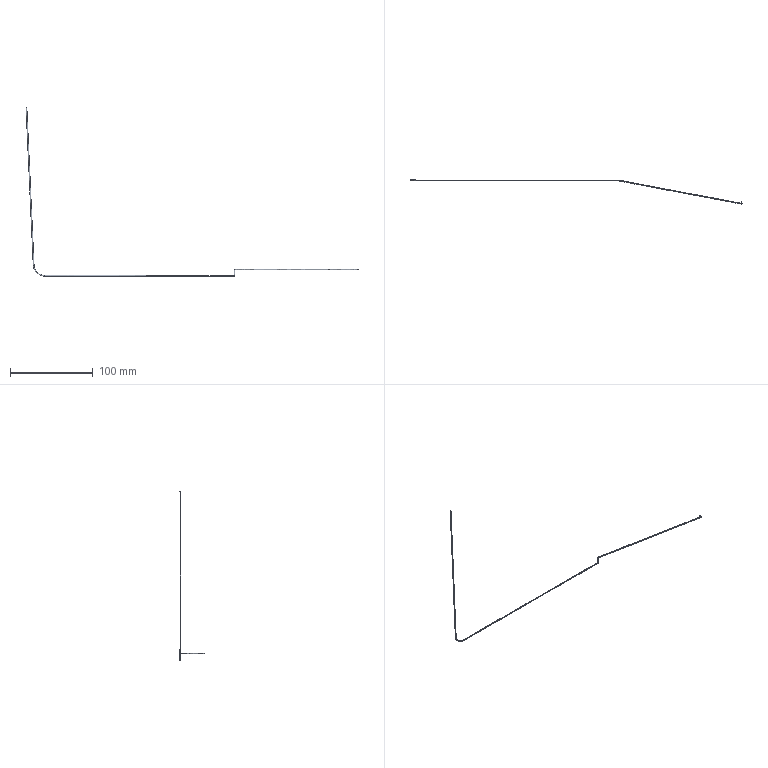Part | SolidWorks | features 3DProfileFeature 4, Sweep 1 | 1 solid | 14 faces | box 401.907 x 29.216 x 204.55 mm | volume 473.935 mm3 | spline 12 | plane 2
STEP:
#1=CARTESIAN_POINT('',(-84.907,75.023,0.4908));
#2=VERTEX_POINT('',#1);
#3=CARTESIAN_POINT('',(-85.093,74.977,-0.4908));
#4=VERTEX_POINT('',#3);
#5=CARTESIAN_POINT('',(-85.,75.,0.));
#6=DIRECTION('',(0.008513,-0.9989,0.04512));
#7=DIRECTION('',(0.1852,0.04591,0.9816));
#8=AXIS2_PLACEMENT_3D('',#5,#6,#7);
#9=CIRCLE('',#8,0.5);
#10=EDGE_CURVE('',#2,#4,#9,.T.);
#11=ORIENTED_EDGE('',*,*,#10,.T.);
#12=CARTESIAN_POINT('',(-85.093,71.998,-0.4908));
#13=VERTEX_POINT('',#12);
#14=CARTESIAN_POINT('',(-85.093,74.977,-0.4908));
#15=CARTESIAN_POINT('',(-85.093,71.998,-0.4908));
#16=B_SPLINE_CURVE_WITH_KNOTS('',1,(#14,#15),.UNSPECIFIED.,.F.,.F.,(2,2),(0.,0.6385),.UNSPECIFIED.);
#17=EDGE_CURVE('',#4,#13,#16,.T.);
#18=ORIENTED_EDGE('',*,*,#17,.T.);
#19=CARTESIAN_POINT('',(-84.907,71.775,0.4908));
#20=VERTEX_POINT('',#19);
#21=CARTESIAN_POINT('',(-85.093,71.998,-0.4908));
#22=CARTESIAN_POINT('',(-85.147,72.063,-0.4806));
#23=CARTESIAN_POINT('',(-85.199,72.127,-0.4617));
#24=CARTESIAN_POINT('',(-85.3,72.248,-0.4037));
#25=CARTESIAN_POINT('',(-85.349,72.307,-0.3639));
#26=CARTESIAN_POINT('',(-85.434,72.41,-0.2574));
#27=CARTESIAN_POINT('',(-85.47,72.454,-0.1886));
#28=CARTESIAN_POINT('',(-85.506,72.497,-0.02785));
#29=CARTESIAN_POINT('',(-85.502,72.492,0.06372));
#30=CARTESIAN_POINT('',(-85.457,72.437,0.2187));
#31=CARTESIAN_POINT('',(-85.418,72.39,0.2827));
#32=CARTESIAN_POINT('',(-85.33,72.284,0.3816));
#33=CARTESIAN_POINT('',(-85.28,72.224,0.4182));
#34=CARTESIAN_POINT('',(-85.126,72.038,0.4971));
#35=CARTESIAN_POINT('',(-85.015,71.905,0.5112));
#36=CARTESIAN_POINT('',(-84.907,71.775,0.4908));
#37=B_SPLINE_CURVE_WITH_KNOTS('',3,(#21,#22,#23,#24,#25,#26,#27,#28,#29,#30,#31,#32,#33,#34,#35,#36),.UNSPECIFIED.,.F.,.F.,(4,2,2,2,2,2,2,4),(0.002044,0.0023,0.002555,0.002811,0.003067,0.003322,0.003578,0.004089),.UNSPECIFIED.);
#38=EDGE_CURVE('',#13,#20,#37,.T.);
#39=ORIENTED_EDGE('',*,*,#38,.T.);
#40=CARTESIAN_POINT('',(-84.907,75.023,0.4908));
#41=CARTESIAN_POINT('',(-84.907,71.775,0.4908));
#42=B_SPLINE_CURVE_WITH_KNOTS('',1,(#40,#41),.UNSPECIFIED.,.F.,.F.,(2,2),(0.,0.6962),.UNSPECIFIED.);
#43=EDGE_CURVE('',#2,#20,#42,.T.);
#44=ORIENTED_EDGE('',*,*,#43,.F.);
#45=EDGE_LOOP('',(#11,#18,#39,#44));
#46=FACE_OUTER_BOUND('',#45,.T.);
#47=CARTESIAN_POINT('',(-84.907,75.023,0.4908));
#48=CARTESIAN_POINT('',(-84.907,70.357,0.4908));
#49=CARTESIAN_POINT('',(-85.89,75.023,0.6762));
#50=CARTESIAN_POINT('',(-85.89,70.357,0.6762));
#51=CARTESIAN_POINT('',(-86.075,74.977,-0.3054));
#52=CARTESIAN_POINT('',(-86.075,70.311,-0.3054));
#53=CARTESIAN_POINT('',(-85.093,74.977,-0.4908));
#54=CARTESIAN_POINT('',(-85.093,70.311,-0.4908));
#55=CARTESIAN_POINT('',(-84.11,74.977,-0.6762));
#56=CARTESIAN_POINT('',(-84.11,70.311,-0.6762));
#57=CARTESIAN_POINT('',(-83.925,75.023,0.3054));
#58=CARTESIAN_POINT('',(-83.925,70.357,0.3054));
#59=CARTESIAN_POINT('',(-84.907,75.023,0.4908));
#60=CARTESIAN_POINT('',(-84.907,70.357,0.4908));
#61=(BOUNDED_SURFACE()B_SPLINE_SURFACE(3,1,((#47,#48),(#49,#50),(#51,#52),(#53,#54),(#55,#56),(#57,#58),(#59,#60)),.UNSPECIFIED.,.T.,.F.,.T.)B_SPLINE_SURFACE_WITH_KNOTS((4,3,4),(2,2),(0.,0.5,1.),(0.,1.),.UNSPECIFIED.)GEOMETRIC_REPRESENTATION_ITEM()RATIONAL_B_SPLINE_SURFACE(((1.,1.),(0.3333,0.3333),(0.3333,0.3333),(1.,1.),(0.3333,0.3333),(0.3333,0.3333),(1.,1.)))REPRESENTATION_ITEM('')SURFACE());
#62=ADVANCED_FACE('',(#46),#61,.T.);
#63=ORIENTED_EDGE('',*,*,#38,.F.);
#64=CARTESIAN_POINT('',(-233.501,100.,-0.4908));
#65=VERTEX_POINT('',#64);
#66=CARTESIAN_POINT('',(-85.093,71.998,-0.4908));
#67=CARTESIAN_POINT('',(-233.501,100.,-0.4908));
#68=B_SPLINE_CURVE_WITH_KNOTS('',1,(#66,#67),.UNSPECIFIED.,.F.,.F.,(2,2),(0.01033,0.991),.UNSPECIFIED.);
#69=EDGE_CURVE('',#13,#65,#68,.T.);
#70=ORIENTED_EDGE('',*,*,#69,.T.);
#71=CARTESIAN_POINT('',(-234.499,100.,0.4908));
#72=VERTEX_POINT('',#71);
#73=CARTESIAN_POINT('',(-233.501,100.,-0.4908));
#74=CARTESIAN_POINT('',(-233.501,100.078,-0.4763));
#75=CARTESIAN_POINT('',(-233.52,100.153,-0.4438));
#76=CARTESIAN_POINT('',(-233.578,100.277,-0.3631));
#77=CARTESIAN_POINT('',(-233.618,100.328,-0.3145));
#78=CARTESIAN_POINT('',(-233.751,100.45,-0.1609));
#79=CARTESIAN_POINT('',(-233.86,100.493,-0.04587));
#80=CARTESIAN_POINT('',(-234.03,100.502,0.1222));
#81=CARTESIAN_POINT('',(-234.086,100.496,0.1766));
#82=CARTESIAN_POINT('',(-234.199,100.462,0.2817));
#83=CARTESIAN_POINT('',(-234.256,100.434,0.3323));
#84=CARTESIAN_POINT('',(-234.361,100.352,0.4199));
#85=CARTESIAN_POINT('',(-234.409,100.297,0.4572));
#86=CARTESIAN_POINT('',(-234.479,100.16,0.5007));
#87=CARTESIAN_POINT('',(-234.499,100.079,0.5055));
#88=CARTESIAN_POINT('',(-234.499,100.,0.4908));
#89=B_SPLINE_CURVE_WITH_KNOTS('',3,(#73,#74,#75,#76,#77,#78,#79,#80,#81,#82,#83,#84,#85,#86,#87,#88),.UNSPECIFIED.,.F.,.F.,(4,2,2,2,2,2,2,4),(0.001901,0.002138,0.002375,0.00285,0.003087,0.003324,0.003562,0.003799),.UNSPECIFIED.);
#90=EDGE_CURVE('',#65,#72,#89,.T.);
#91=ORIENTED_EDGE('',*,*,#90,.T.);
#92=CARTESIAN_POINT('',(-84.907,71.775,0.4908));
#93=CARTESIAN_POINT('',(-234.499,100.,0.4908));
#94=B_SPLINE_CURVE_WITH_KNOTS('',1,(#92,#93),.UNSPECIFIED.,.F.,.F.,(2,2),(0.009174,0.9977),.UNSPECIFIED.);
#95=EDGE_CURVE('',#20,#72,#94,.T.);
#96=ORIENTED_EDGE('',*,*,#95,.F.);
#97=EDGE_LOOP('',(#63,#70,#91,#96));
#98=FACE_OUTER_BOUND('',#97,.T.);
#99=CARTESIAN_POINT('',(-83.519,71.513,0.4908));
#100=CARTESIAN_POINT('',(-234.849,100.066,0.4908));
#101=CARTESIAN_POINT('',(-83.337,72.478,0.6762));
#102=CARTESIAN_POINT('',(-234.666,101.032,0.6762));
#103=CARTESIAN_POINT('',(-83.348,72.669,-0.3054));
#104=CARTESIAN_POINT('',(-234.677,101.222,-0.3054));
#105=CARTESIAN_POINT('',(-83.53,71.703,-0.4908));
#106=CARTESIAN_POINT('',(-234.859,100.256,-0.4908));
#107=CARTESIAN_POINT('',(-83.712,70.738,-0.6762));
#108=CARTESIAN_POINT('',(-235.042,99.291,-0.6762));
#109=CARTESIAN_POINT('',(-83.701,70.547,0.3054));
#110=CARTESIAN_POINT('',(-235.031,99.1,0.3054));
#111=CARTESIAN_POINT('',(-83.519,71.513,0.4908));
#112=CARTESIAN_POINT('',(-234.849,100.066,0.4908));
#113=(BOUNDED_SURFACE()B_SPLINE_SURFACE(3,1,((#99,#100),(#101,#102),(#103,#104),(#105,#106),(#107,#108),(#109,#110),(#111,#112)),.UNSPECIFIED.,.T.,.F.,.F.)B_SPLINE_SURFACE_WITH_KNOTS((4,3,4),(2,2),(0.,0.5,1.),(0.,1.),.UNSPECIFIED.)GEOMETRIC_REPRESENTATION_ITEM()RATIONAL_B_SPLINE_SURFACE(((1.,1.),(0.3333,0.3333),(0.3333,0.3333),(1.,1.),(0.3333,0.3333),(0.3333,0.3333),(1.,1.)))REPRESENTATION_ITEM('')SURFACE());
#114=ADVANCED_FACE('',(#98),#113,.T.);
#115=ORIENTED_EDGE('',*,*,#90,.F.);
#116=CARTESIAN_POINT('',(-233.501,100.,-8.501));
#117=VERTEX_POINT('',#116);
#118=CARTESIAN_POINT('',(-233.501,100.,-0.4908));
#119=CARTESIAN_POINT('',(-233.501,100.,-8.501));
#120=B_SPLINE_CURVE_WITH_KNOTS('',1,(#118,#119),.UNSPECIFIED.,.F.,.F.,(2,2),(0.1362,0.9844),.UNSPECIFIED.);
#121=EDGE_CURVE('',#65,#117,#120,.T.);
#122=ORIENTED_EDGE('',*,*,#121,.T.);
#123=CARTESIAN_POINT('',(-234.499,100.,-7.499));
#124=VERTEX_POINT('',#123);
#125=CARTESIAN_POINT('',(-233.501,100.,-8.501));
#126=CARTESIAN_POINT('',(-233.501,100.079,-8.501));
#127=CARTESIAN_POINT('',(-233.521,100.159,-8.48));
#128=CARTESIAN_POINT('',(-233.586,100.289,-8.415));
#129=CARTESIAN_POINT('',(-233.63,100.342,-8.371));
#130=CARTESIAN_POINT('',(-233.774,100.463,-8.226));
#131=CARTESIAN_POINT('',(-233.888,100.5,-8.112));
#132=CARTESIAN_POINT('',(-234.112,100.5,-7.888));
#133=CARTESIAN_POINT('',(-234.225,100.464,-7.775));
#134=CARTESIAN_POINT('',(-234.371,100.341,-7.629));
#135=CARTESIAN_POINT('',(-234.414,100.288,-7.585));
#136=CARTESIAN_POINT('',(-234.479,100.158,-7.52));
#137=CARTESIAN_POINT('',(-234.499,100.081,-7.499));
#138=CARTESIAN_POINT('',(-234.499,100.,-7.499));
#139=B_SPLINE_CURVE_WITH_KNOTS('',3,(#125,#126,#127,#128,#129,#130,#131,#132,#133,#134,#135,#136,#137,#138),.UNSPECIFIED.,.F.,.F.,(4,2,2,2,2,2,4),(0.001905,0.002143,0.002381,0.002857,0.003333,0.003571,0.003809),.UNSPECIFIED.);
#140=EDGE_CURVE('',#117,#124,#139,.T.);
#141=ORIENTED_EDGE('',*,*,#140,.T.);
#142=CARTESIAN_POINT('',(-234.499,100.,0.4908));
#143=CARTESIAN_POINT('',(-234.499,100.,-7.499));
#144=B_SPLINE_CURVE_WITH_KNOTS('',1,(#142,#143),.UNSPECIFIED.,.F.,.F.,(2,2),(0.03714,0.8832),.UNSPECIFIED.);
#145=EDGE_CURVE('',#72,#124,#144,.T.);
#146=ORIENTED_EDGE('',*,*,#145,.F.);
#147=EDGE_LOOP('',(#115,#122,#141,#146));
#148=FACE_OUTER_BOUND('',#147,.T.);
#149=CARTESIAN_POINT('',(-234.499,100.,0.8415));
#150=CARTESIAN_POINT('',(-234.499,100.,-8.602));
#151=CARTESIAN_POINT('',(-234.499,101.,0.8415));
#152=CARTESIAN_POINT('',(-234.499,101.,-8.602));
#153=CARTESIAN_POINT('',(-233.501,101.,0.7956));
#154=CARTESIAN_POINT('',(-233.501,101.,-8.648));
#155=CARTESIAN_POINT('',(-233.501,100.,0.7956));
#156=CARTESIAN_POINT('',(-233.501,100.,-8.648));
#157=CARTESIAN_POINT('',(-233.501,99.,0.7956));
#158=CARTESIAN_POINT('',(-233.501,99.,-8.648));
#159=CARTESIAN_POINT('',(-234.499,99.,0.8415));
#160=CARTESIAN_POINT('',(-234.499,99.,-8.602));
#161=CARTESIAN_POINT('',(-234.499,100.,0.8415));
#162=CARTESIAN_POINT('',(-234.499,100.,-8.602));
#163=(BOUNDED_SURFACE()B_SPLINE_SURFACE(3,1,((#149,#150),(#151,#152),(#153,#154),(#155,#156),(#157,#158),(#159,#160),(#161,#162)),.UNSPECIFIED.,.T.,.F.,.T.)B_SPLINE_SURFACE_WITH_KNOTS((4,3,4),(2,2),(0.,0.5,1.),(0.,1.),.UNSPECIFIED.)GEOMETRIC_REPRESENTATION_ITEM()RATIONAL_B_SPLINE_SURFACE(((1.,1.),(0.3333,0.3333),(0.3333,0.3333),(1.,1.),(0.3333,0.3333),(0.3333,0.3333),(1.,1.)))REPRESENTATION_ITEM('')SURFACE());
#164=ADVANCED_FACE('',(#148),#163,.T.);
#165=CARTESIAN_POINT('',(-476.621,100.,4.881));
#166=VERTEX_POINT('',#165);
#167=CARTESIAN_POINT('',(-477.621,100.,4.881));
#168=VERTEX_POINT('',#167);
#169=CARTESIAN_POINT('',(-477.121,100.,4.881));
#170=DIRECTION('',(0.,0.,1.));
#171=DIRECTION('',(1.,0.,0.));
#172=AXIS2_PLACEMENT_3D('',#169,#170,#171);
#173=CIRCLE('',#172,0.5);
#174=EDGE_CURVE('',#166,#168,#173,.T.);
#175=ORIENTED_EDGE('',*,*,#174,.T.);
#176=CARTESIAN_POINT('',(-486.407,100.,196.049));
#177=VERTEX_POINT('',#176);
#178=CARTESIAN_POINT('',(-477.621,100.,4.881));
#179=CARTESIAN_POINT('',(-486.407,100.,196.049));
#180=B_SPLINE_CURVE_WITH_KNOTS('',1,(#178,#179),.UNSPECIFIED.,.F.,.F.,(2,2),(0.,1.),.UNSPECIFIED.);
#181=EDGE_CURVE('',#168,#177,#180,.T.);
#182=ORIENTED_EDGE('',*,*,#181,.T.);
#183=CARTESIAN_POINT('',(-485.407,100.,196.049));
#184=VERTEX_POINT('',#183);
#185=CARTESIAN_POINT('',(-485.907,100.,196.049));
#186=DIRECTION('',(0.,0.,1.));
#187=DIRECTION('',(1.,0.,0.));
#188=AXIS2_PLACEMENT_3D('',#185,#186,#187);
#189=CIRCLE('',#188,0.5);
#190=EDGE_CURVE('',#184,#177,#189,.T.);
#191=ORIENTED_EDGE('',*,*,#190,.F.);
#192=CARTESIAN_POINT('',(-476.621,100.,4.881));
#193=CARTESIAN_POINT('',(-485.407,100.,196.049));
#194=B_SPLINE_CURVE_WITH_KNOTS('',1,(#192,#193),.UNSPECIFIED.,.F.,.F.,(2,2),(0.,1.),.UNSPECIFIED.);
#195=EDGE_CURVE('',#166,#184,#194,.T.);
#196=ORIENTED_EDGE('',*,*,#195,.F.);
#197=EDGE_LOOP('',(#175,#182,#191,#196));
#198=FACE_OUTER_BOUND('',#197,.T.);
#199=CARTESIAN_POINT('',(-476.621,100.,4.881));
#200=CARTESIAN_POINT('',(-485.407,100.,196.049));
#201=CARTESIAN_POINT('',(-476.621,101.,4.881));
#202=CARTESIAN_POINT('',(-485.407,101.,196.049));
#203=CARTESIAN_POINT('',(-477.621,101.,4.881));
#204=CARTESIAN_POINT('',(-486.407,101.,196.049));
#205=CARTESIAN_POINT('',(-477.621,100.,4.881));
#206=CARTESIAN_POINT('',(-486.407,100.,196.049));
#207=CARTESIAN_POINT('',(-477.621,99.,4.881));
#208=CARTESIAN_POINT('',(-486.407,99.,196.049));
#209=CARTESIAN_POINT('',(-476.621,99.,4.881));
#210=CARTESIAN_POINT('',(-485.407,99.,196.049));
#211=CARTESIAN_POINT('',(-476.621,100.,4.881));
#212=CARTESIAN_POINT('',(-485.407,100.,196.049));
#213=(BOUNDED_SURFACE()B_SPLINE_SURFACE(3,1,((#199,#200),(#201,#202),(#203,#204),(#205,#206),(#207,#208),(#209,#210),(#211,#212)),.UNSPECIFIED.,.T.,.F.,.F.)B_SPLINE_SURFACE_WITH_KNOTS((4,3,4),(2,2),(0.,0.5,1.),(0.,1.),.UNSPECIFIED.)GEOMETRIC_REPRESENTATION_ITEM()RATIONAL_B_SPLINE_SURFACE(((1.,1.),(0.3333,0.3333),(0.3333,0.3333),(1.,1.),(0.3333,0.3333),(0.3333,0.3333),(1.,1.)))REPRESENTATION_ITEM('')SURFACE());
#214=ADVANCED_FACE('',(#198),#213,.T.);
#215=CARTESIAN_POINT('',(-464.137,100.,-7.023));
#216=VERTEX_POINT('',#215);
#217=CARTESIAN_POINT('',(-464.185,100.,-8.021));
#218=VERTEX_POINT('',#217);
#219=CARTESIAN_POINT('',(-464.161,100.,-7.522));
#220=DIRECTION('',(-0.9988,0.,0.04799));
#221=DIRECTION('',(0.04799,0.,0.9988));
#222=AXIS2_PLACEMENT_3D('',#219,#220,#221);
#223=CIRCLE('',#222,0.5);
#224=EDGE_CURVE('',#216,#218,#223,.T.);
#225=ORIENTED_EDGE('',*,*,#224,.T.);
#226=CARTESIAN_POINT('',(-464.185,100.,-8.021));
#227=CARTESIAN_POINT('',(-471.795,100.,-7.993));
#228=CARTESIAN_POINT('',(-477.284,100.,-2.721));
#229=CARTESIAN_POINT('',(-477.621,100.,4.881));
#230=(BOUNDED_CURVE()B_SPLINE_CURVE(3,(#226,#227,#228,#229),.UNSPECIFIED.,.F.,.F.)B_SPLINE_CURVE_WITH_KNOTS((4,4),(0.,1.),.UNSPECIFIED.)CURVE()GEOMETRIC_REPRESENTATION_ITEM()RATIONAL_B_SPLINE_CURVE((1.,0.8159,0.8159,1.))REPRESENTATION_ITEM(''));
#231=EDGE_CURVE('',#218,#168,#230,.T.);
#232=ORIENTED_EDGE('',*,*,#231,.T.);
#233=ORIENTED_EDGE('',*,*,#174,.F.);
#234=CARTESIAN_POINT('',(-464.137,100.,-7.023));
#235=CARTESIAN_POINT('',(-471.184,100.,-7.021));
#236=CARTESIAN_POINT('',(-476.284,100.,-2.158));
#237=CARTESIAN_POINT('',(-476.621,100.,4.881));
#238=(BOUNDED_CURVE()B_SPLINE_CURVE(3,(#234,#235,#236,#237),.UNSPECIFIED.,.F.,.F.)B_SPLINE_CURVE_WITH_KNOTS((4,4),(0.,1.),.UNSPECIFIED.)CURVE()GEOMETRIC_REPRESENTATION_ITEM()RATIONAL_B_SPLINE_CURVE((1.,0.8159,0.8159,1.))REPRESENTATION_ITEM(''));
#239=EDGE_CURVE('',#216,#166,#238,.T.);
#240=ORIENTED_EDGE('',*,*,#239,.F.);
#241=EDGE_LOOP('',(#225,#232,#233,#240));
#242=FACE_OUTER_BOUND('',#241,.T.);
#243=CARTESIAN_POINT('',(-464.137,100.,-7.023));
#244=CARTESIAN_POINT('',(-471.184,100.,-7.021));
#245=CARTESIAN_POINT('',(-476.284,100.,-2.158));
#246=CARTESIAN_POINT('',(-476.621,100.,4.881));
#247=CARTESIAN_POINT('',(-464.137,101.,-7.023));
#248=CARTESIAN_POINT('',(-471.184,101.,-7.021));
#249=CARTESIAN_POINT('',(-476.284,101.,-2.158));
#250=CARTESIAN_POINT('',(-476.621,101.,4.881));
#251=CARTESIAN_POINT('',(-464.185,101.,-8.021));
#252=CARTESIAN_POINT('',(-471.795,101.,-7.993));
#253=CARTESIAN_POINT('',(-477.284,101.,-2.721));
#254=CARTESIAN_POINT('',(-477.621,101.,4.881));
#255=CARTESIAN_POINT('',(-464.185,100.,-8.021));
#256=CARTESIAN_POINT('',(-471.795,100.,-7.993));
#257=CARTESIAN_POINT('',(-477.284,100.,-2.721));
#258=CARTESIAN_POINT('',(-477.621,100.,4.881));
#259=CARTESIAN_POINT('',(-464.185,99.,-8.021));
#260=CARTESIAN_POINT('',(-471.795,99.,-7.993));
#261=CARTESIAN_POINT('',(-477.284,99.,-2.721));
#262=CARTESIAN_POINT('',(-477.621,99.,4.881));
#263=CARTESIAN_POINT('',(-464.137,99.,-7.023));
#264=CARTESIAN_POINT('',(-471.184,99.,-7.021));
#265=CARTESIAN_POINT('',(-476.284,99.,-2.158));
#266=CARTESIAN_POINT('',(-476.621,99.,4.881));
#267=CARTESIAN_POINT('',(-464.137,100.,-7.023));
#268=CARTESIAN_POINT('',(-471.184,100.,-7.021));
#269=CARTESIAN_POINT('',(-476.284,100.,-2.158));
#270=CARTESIAN_POINT('',(-476.621,100.,4.881));
#271=(BOUNDED_SURFACE()B_SPLINE_SURFACE(3,3,((#243,#244,#245,#246),(#247,#248,#249,#250),(#251,#252,#253,#254),(#255,#256,#257,#258),(#259,#260,#261,#262),(#263,#264,#265,#266),(#267,#268,#269,#270)),.UNSPECIFIED.,.T.,.F.,.F.)B_SPLINE_SURFACE_WITH_KNOTS((4,3,4),(4,4),(0.,0.5,1.),(0.,1.),.UNSPECIFIED.)GEOMETRIC_REPRESENTATION_ITEM()RATIONAL_B_SPLINE_SURFACE(((1.,0.8159,0.8159,1.),(0.3333,0.272,0.272,0.3333),(0.3333,0.272,0.272,0.3333),(1.,0.8159,0.8159,1.),(0.3333,0.272,0.272,0.3333),(0.3333,0.272,0.272,0.3333),(1.,0.8159,0.8159,1.)))REPRESENTATION_ITEM('')SURFACE());
#272=ADVANCED_FACE('',(#242),#271,.T.);
#273=ORIENTED_EDGE('',*,*,#140,.F.);
#274=CARTESIAN_POINT('',(-233.501,100.,-8.501));
#275=CARTESIAN_POINT('',(-464.185,100.,-8.021));
#276=B_SPLINE_CURVE_WITH_KNOTS('',1,(#274,#275),.UNSPECIFIED.,.F.,.F.,(2,2),(0.00066,1.),.UNSPECIFIED.);
#277=EDGE_CURVE('',#117,#218,#276,.T.);
#278=ORIENTED_EDGE('',*,*,#277,.T.);
#279=ORIENTED_EDGE('',*,*,#224,.F.);
#280=CARTESIAN_POINT('',(-234.499,100.,-7.499));
#281=CARTESIAN_POINT('',(-464.137,100.,-7.023));
#282=B_SPLINE_CURVE_WITH_KNOTS('',1,(#280,#281),.UNSPECIFIED.,.F.,.F.,(2,2),(0.005195,1.),.UNSPECIFIED.);
#283=EDGE_CURVE('',#124,#216,#282,.T.);
#284=ORIENTED_EDGE('',*,*,#283,.F.);
#285=EDGE_LOOP('',(#273,#278,#279,#284));
#286=FACE_OUTER_BOUND('',#285,.T.);
#287=CARTESIAN_POINT('',(-233.3,100.,-7.502));
#288=CARTESIAN_POINT('',(-464.137,100.,-7.023));
#289=CARTESIAN_POINT('',(-233.3,101.,-7.502));
#290=CARTESIAN_POINT('',(-464.137,101.,-7.023));
#291=CARTESIAN_POINT('',(-233.348,101.,-8.501));
#292=CARTESIAN_POINT('',(-464.185,101.,-8.021));
#293=CARTESIAN_POINT('',(-233.348,100.,-8.501));
#294=CARTESIAN_POINT('',(-464.185,100.,-8.021));
#295=CARTESIAN_POINT('',(-233.348,99.,-8.501));
#296=CARTESIAN_POINT('',(-464.185,99.,-8.021));
#297=CARTESIAN_POINT('',(-233.3,99.,-7.502));
#298=CARTESIAN_POINT('',(-464.137,99.,-7.023));
#299=CARTESIAN_POINT('',(-233.3,100.,-7.502));
#300=CARTESIAN_POINT('',(-464.137,100.,-7.023));
#301=(BOUNDED_SURFACE()B_SPLINE_SURFACE(3,1,((#287,#288),(#289,#290),(#291,#292),(#293,#294),(#295,#296),(#297,#298),(#299,#300)),.UNSPECIFIED.,.T.,.F.,.T.)B_SPLINE_SURFACE_WITH_KNOTS((4,3,4),(2,2),(0.,0.5,1.),(0.,1.),.UNSPECIFIED.)GEOMETRIC_REPRESENTATION_ITEM()RATIONAL_B_SPLINE_SURFACE(((1.,1.),(0.3333,0.3333),(0.3333,0.3333),(1.,1.),(0.3333,0.3333),(0.3333,0.3333),(1.,1.)))REPRESENTATION_ITEM('')SURFACE());
#302=ADVANCED_FACE('',(#286),#301,.T.);
#303=ORIENTED_EDGE('',*,*,#17,.F.);
#304=CARTESIAN_POINT('',(-85.,75.,0.));
#305=DIRECTION('',(0.008513,-0.9989,0.04512));
#306=DIRECTION('',(0.1852,0.04591,0.9816));
#307=AXIS2_PLACEMENT_3D('',#304,#305,#306);
#308=CIRCLE('',#307,0.5);
#309=EDGE_CURVE('',#4,#2,#308,.T.);
#310=ORIENTED_EDGE('',*,*,#309,.T.);
#311=ORIENTED_EDGE('',*,*,#43,.T.);
#312=CARTESIAN_POINT('',(-84.907,71.775,0.4908));
#313=CARTESIAN_POINT('',(-84.853,71.709,0.4806));
#314=CARTESIAN_POINT('',(-84.8,71.645,0.4614));
#315=CARTESIAN_POINT('',(-84.699,71.523,0.403));
#316=CARTESIAN_POINT('',(-84.65,71.465,0.3633));
#317=CARTESIAN_POINT('',(-84.566,71.363,0.2566));
#318=CARTESIAN_POINT('',(-84.53,71.319,0.1883));
#319=CARTESIAN_POINT('',(-84.494,71.276,0.02653));
#320=CARTESIAN_POINT('',(-84.498,71.28,-0.06461));
#321=CARTESIAN_POINT('',(-84.543,71.336,-0.2193));
#322=CARTESIAN_POINT('',(-84.583,71.383,-0.283));
#323=CARTESIAN_POINT('',(-84.671,71.49,-0.3821));
#324=CARTESIAN_POINT('',(-84.72,71.549,-0.4182));
#325=CARTESIAN_POINT('',(-84.875,71.736,-0.4974));
#326=CARTESIAN_POINT('',(-84.985,71.868,-0.5112));
#327=CARTESIAN_POINT('',(-85.093,71.998,-0.4908));
#328=B_SPLINE_CURVE_WITH_KNOTS('',3,(#312,#313,#314,#315,#316,#317,#318,#319,#320,#321,#322,#323,#324,#325,#326,#327),.UNSPECIFIED.,.F.,.F.,(4,2,2,2,2,2,2,4),(0.,0.0002555,0.0005111,0.0007666,0.001022,0.001278,0.001533,0.002044),.UNSPECIFIED.);
#329=EDGE_CURVE('',#20,#13,#328,.T.);
#330=ORIENTED_EDGE('',*,*,#329,.T.);
#331=EDGE_LOOP('',(#303,#310,#311,#330));
#332=FACE_OUTER_BOUND('',#331,.T.);
#333=CARTESIAN_POINT('',(-84.907,75.023,0.4908));
#334=CARTESIAN_POINT('',(-84.907,70.357,0.4908));
#335=CARTESIAN_POINT('',(-85.89,75.023,0.6762));
#336=CARTESIAN_POINT('',(-85.89,70.357,0.6762));
#337=CARTESIAN_POINT('',(-86.075,74.977,-0.3054));
#338=CARTESIAN_POINT('',(-86.075,70.311,-0.3054));
#339=CARTESIAN_POINT('',(-85.093,74.977,-0.4908));
#340=CARTESIAN_POINT('',(-85.093,70.311,-0.4908));
#341=CARTESIAN_POINT('',(-84.11,74.977,-0.6762));
#342=CARTESIAN_POINT('',(-84.11,70.311,-0.6762));
#343=CARTESIAN_POINT('',(-83.925,75.023,0.3054));
#344=CARTESIAN_POINT('',(-83.925,70.357,0.3054));
#345=CARTESIAN_POINT('',(-84.907,75.023,0.4908));
#346=CARTESIAN_POINT('',(-84.907,70.357,0.4908));
#347=(BOUNDED_SURFACE()B_SPLINE_SURFACE(3,1,((#333,#334),(#335,#336),(#337,#338),(#339,#340),(#341,#342),(#343,#344),(#345,#346)),.UNSPECIFIED.,.T.,.F.,.T.)B_SPLINE_SURFACE_WITH_KNOTS((4,3,4),(2,2),(0.,0.5,1.),(0.,1.),.UNSPECIFIED.)GEOMETRIC_REPRESENTATION_ITEM()RATIONAL_B_SPLINE_SURFACE(((1.,1.),(0.3333,0.3333),(0.3333,0.3333),(1.,1.),(0.3333,0.3333),(0.3333,0.3333),(1.,1.)))REPRESENTATION_ITEM('')SURFACE());
#348=ADVANCED_FACE('',(#332),#347,.T.);
#349=ORIENTED_EDGE('',*,*,#69,.F.);
#350=ORIENTED_EDGE('',*,*,#329,.F.);
#351=ORIENTED_EDGE('',*,*,#95,.T.);
#352=CARTESIAN_POINT('',(-234.499,100.,0.4908));
#353=CARTESIAN_POINT('',(-234.499,99.921,0.4761));
#354=CARTESIAN_POINT('',(-234.481,99.848,0.4441));
#355=CARTESIAN_POINT('',(-234.422,99.724,0.3634));
#356=CARTESIAN_POINT('',(-234.382,99.672,0.3149));
#357=CARTESIAN_POINT('',(-234.249,99.55,0.1608));
#358=CARTESIAN_POINT('',(-234.139,99.507,0.04545));
#359=CARTESIAN_POINT('',(-233.915,99.495,-0.1772));
#360=CARTESIAN_POINT('',(-233.796,99.524,-0.2886));
#361=CARTESIAN_POINT('',(-233.639,99.648,-0.4203));
#362=CARTESIAN_POINT('',(-233.591,99.704,-0.4573));
#363=CARTESIAN_POINT('',(-233.521,99.84,-0.5007));
#364=CARTESIAN_POINT('',(-233.501,99.922,-0.5053));
#365=CARTESIAN_POINT('',(-233.501,100.,-0.4908));
#366=B_SPLINE_CURVE_WITH_KNOTS('',3,(#352,#353,#354,#355,#356,#357,#358,#359,#360,#361,#362,#363,#364,#365),.UNSPECIFIED.,.F.,.F.,(4,2,2,2,2,2,4),(0.,0.0002376,0.0004752,0.0009503,0.001425,0.001663,0.001901),.UNSPECIFIED.);
#367=EDGE_CURVE('',#72,#65,#366,.T.);
#368=ORIENTED_EDGE('',*,*,#367,.T.);
#369=EDGE_LOOP('',(#349,#350,#351,#368));
#370=FACE_OUTER_BOUND('',#369,.T.);
#371=CARTESIAN_POINT('',(-83.519,71.513,0.4908));
#372=CARTESIAN_POINT('',(-234.849,100.066,0.4908));
#373=CARTESIAN_POINT('',(-83.337,72.478,0.6762));
#374=CARTESIAN_POINT('',(-234.666,101.032,0.6762));
#375=CARTESIAN_POINT('',(-83.348,72.669,-0.3054));
#376=CARTESIAN_POINT('',(-234.677,101.222,-0.3054));
#377=CARTESIAN_POINT('',(-83.53,71.703,-0.4908));
#378=CARTESIAN_POINT('',(-234.859,100.256,-0.4908));
#379=CARTESIAN_POINT('',(-83.712,70.738,-0.6762));
#380=CARTESIAN_POINT('',(-235.042,99.291,-0.6762));
#381=CARTESIAN_POINT('',(-83.701,70.547,0.3054));
#382=CARTESIAN_POINT('',(-235.031,99.1,0.3054));
#383=CARTESIAN_POINT('',(-83.519,71.513,0.4908));
#384=CARTESIAN_POINT('',(-234.849,100.066,0.4908));
#385=(BOUNDED_SURFACE()B_SPLINE_SURFACE(3,1,((#371,#372),(#373,#374),(#375,#376),(#377,#378),(#379,#380),(#381,#382),(#383,#384)),.UNSPECIFIED.,.T.,.F.,.T.)B_SPLINE_SURFACE_WITH_KNOTS((4,3,4),(2,2),(0.,0.5,1.),(0.,1.),.UNSPECIFIED.)GEOMETRIC_REPRESENTATION_ITEM()RATIONAL_B_SPLINE_SURFACE(((1.,1.),(0.3333,0.3333),(0.3333,0.3333),(1.,1.),(0.3333,0.3333),(0.3333,0.3333),(1.,1.)))REPRESENTATION_ITEM('')SURFACE());
#386=ADVANCED_FACE('',(#370),#385,.T.);
#387=ORIENTED_EDGE('',*,*,#121,.F.);
#388=ORIENTED_EDGE('',*,*,#367,.F.);
#389=ORIENTED_EDGE('',*,*,#145,.T.);
#390=CARTESIAN_POINT('',(-234.499,100.,-7.499));
#391=CARTESIAN_POINT('',(-234.499,99.919,-7.499));
#392=CARTESIAN_POINT('',(-234.479,99.842,-7.52));
#393=CARTESIAN_POINT('',(-234.414,99.711,-7.585));
#394=CARTESIAN_POINT('',(-234.37,99.658,-7.629));
#395=CARTESIAN_POINT('',(-234.225,99.536,-7.775));
#396=CARTESIAN_POINT('',(-234.112,99.5,-7.888));
#397=CARTESIAN_POINT('',(-233.888,99.5,-8.112));
#398=CARTESIAN_POINT('',(-233.775,99.536,-8.226));
#399=CARTESIAN_POINT('',(-233.63,99.658,-8.371));
#400=CARTESIAN_POINT('',(-233.586,99.711,-8.415));
#401=CARTESIAN_POINT('',(-233.521,99.841,-8.48));
#402=CARTESIAN_POINT('',(-233.501,99.92,-8.501));
#403=CARTESIAN_POINT('',(-233.501,100.,-8.501));
#404=B_SPLINE_CURVE_WITH_KNOTS('',3,(#390,#391,#392,#393,#394,#395,#396,#397,#398,#399,#400,#401,#402,#403),.UNSPECIFIED.,.F.,.F.,(4,2,2,2,2,2,4),(0.,0.0002381,0.0004763,0.0009525,0.001429,0.001667,0.001905),.UNSPECIFIED.);
#405=EDGE_CURVE('',#124,#117,#404,.T.);
#406=ORIENTED_EDGE('',*,*,#405,.T.);
#407=EDGE_LOOP('',(#387,#388,#389,#406));
#408=FACE_OUTER_BOUND('',#407,.T.);
#409=CARTESIAN_POINT('',(-234.499,100.,0.8415));
#410=CARTESIAN_POINT('',(-234.499,100.,-8.602));
#411=CARTESIAN_POINT('',(-234.499,101.,0.8415));
#412=CARTESIAN_POINT('',(-234.499,101.,-8.602));
#413=CARTESIAN_POINT('',(-233.501,101.,0.7956));
#414=CARTESIAN_POINT('',(-233.501,101.,-8.648));
#415=CARTESIAN_POINT('',(-233.501,100.,0.7956));
#416=CARTESIAN_POINT('',(-233.501,100.,-8.648));
#417=CARTESIAN_POINT('',(-233.501,99.,0.7956));
#418=CARTESIAN_POINT('',(-233.501,99.,-8.648));
#419=CARTESIAN_POINT('',(-234.499,99.,0.8415));
#420=CARTESIAN_POINT('',(-234.499,99.,-8.602));
#421=CARTESIAN_POINT('',(-234.499,100.,0.8415));
#422=CARTESIAN_POINT('',(-234.499,100.,-8.602));
#423=(BOUNDED_SURFACE()B_SPLINE_SURFACE(3,1,((#409,#410),(#411,#412),(#413,#414),(#415,#416),(#417,#418),(#419,#420),(#421,#422)),.UNSPECIFIED.,.T.,.F.,.T.)B_SPLINE_SURFACE_WITH_KNOTS((4,3,4),(2,2),(0.,0.5,1.),(0.,1.),.UNSPECIFIED.)GEOMETRIC_REPRESENTATION_ITEM()RATIONAL_B_SPLINE_SURFACE(((1.,1.),(0.3333,0.3333),(0.3333,0.3333),(1.,1.),(0.3333,0.3333),(0.3333,0.3333),(1.,1.)))REPRESENTATION_ITEM('')SURFACE());
#424=ADVANCED_FACE('',(#408),#423,.T.);
#425=ORIENTED_EDGE('',*,*,#181,.F.);
#426=CARTESIAN_POINT('',(-477.121,100.,4.881));
#427=DIRECTION('',(0.,0.,1.));
#428=DIRECTION('',(1.,0.,0.));
#429=AXIS2_PLACEMENT_3D('',#426,#427,#428);
#430=CIRCLE('',#429,0.5);
#431=EDGE_CURVE('',#168,#166,#430,.T.);
#432=ORIENTED_EDGE('',*,*,#431,.T.);
#433=ORIENTED_EDGE('',*,*,#195,.T.);
#434=CARTESIAN_POINT('',(-485.907,100.,196.049));
#435=DIRECTION('',(0.,0.,1.));
#436=DIRECTION('',(1.,0.,0.));
#437=AXIS2_PLACEMENT_3D('',#434,#435,#436);
#438=CIRCLE('',#437,0.5);
#439=EDGE_CURVE('',#177,#184,#438,.T.);
#440=ORIENTED_EDGE('',*,*,#439,.F.);
#441=EDGE_LOOP('',(#425,#432,#433,#440));
#442=FACE_OUTER_BOUND('',#441,.T.);
#443=CARTESIAN_POINT('',(-476.621,100.,4.881));
#444=CARTESIAN_POINT('',(-485.407,100.,196.049));
#445=CARTESIAN_POINT('',(-476.621,101.,4.881));
#446=CARTESIAN_POINT('',(-485.407,101.,196.049));
#447=CARTESIAN_POINT('',(-477.621,101.,4.881));
#448=CARTESIAN_POINT('',(-486.407,101.,196.049));
#449=CARTESIAN_POINT('',(-477.621,100.,4.881));
#450=CARTESIAN_POINT('',(-486.407,100.,196.049));
#451=CARTESIAN_POINT('',(-477.621,99.,4.881));
#452=CARTESIAN_POINT('',(-486.407,99.,196.049));
#453=CARTESIAN_POINT('',(-476.621,99.,4.881));
#454=CARTESIAN_POINT('',(-485.407,99.,196.049));
#455=CARTESIAN_POINT('',(-476.621,100.,4.881));
#456=CARTESIAN_POINT('',(-485.407,100.,196.049));
#457=(BOUNDED_SURFACE()B_SPLINE_SURFACE(3,1,((#443,#444),(#445,#446),(#447,#448),(#449,#450),(#451,#452),(#453,#454),(#455,#456)),.UNSPECIFIED.,.T.,.F.,.F.)B_SPLINE_SURFACE_WITH_KNOTS((4,3,4),(2,2),(0.,0.5,1.),(0.,1.),.UNSPECIFIED.)GEOMETRIC_REPRESENTATION_ITEM()RATIONAL_B_SPLINE_SURFACE(((1.,1.),(0.3333,0.3333),(0.3333,0.3333),(1.,1.),(0.3333,0.3333),(0.3333,0.3333),(1.,1.)))REPRESENTATION_ITEM('')SURFACE());
#458=ADVANCED_FACE('',(#442),#457,.T.);
#459=ORIENTED_EDGE('',*,*,#231,.F.);
#460=CARTESIAN_POINT('',(-464.161,100.,-7.522));
#461=DIRECTION('',(-0.9988,0.,0.04799));
#462=DIRECTION('',(0.04799,0.,0.9988));
#463=AXIS2_PLACEMENT_3D('',#460,#461,#462);
#464=CIRCLE('',#463,0.5);
#465=EDGE_CURVE('',#218,#216,#464,.T.);
#466=ORIENTED_EDGE('',*,*,#465,.T.);
#467=ORIENTED_EDGE('',*,*,#239,.T.);
#468=ORIENTED_EDGE('',*,*,#431,.F.);
#469=EDGE_LOOP('',(#459,#466,#467,#468));
#470=FACE_OUTER_BOUND('',#469,.T.);
#471=CARTESIAN_POINT('',(-464.137,100.,-7.023));
#472=CARTESIAN_POINT('',(-471.184,100.,-7.021));
#473=CARTESIAN_POINT('',(-476.284,100.,-2.158));
#474=CARTESIAN_POINT('',(-476.621,100.,4.881));
#475=CARTESIAN_POINT('',(-464.137,101.,-7.023));
#476=CARTESIAN_POINT('',(-471.184,101.,-7.021));
#477=CARTESIAN_POINT('',(-476.284,101.,-2.158));
#478=CARTESIAN_POINT('',(-476.621,101.,4.881));
#479=CARTESIAN_POINT('',(-464.185,101.,-8.021));
#480=CARTESIAN_POINT('',(-471.795,101.,-7.993));
#481=CARTESIAN_POINT('',(-477.284,101.,-2.721));
#482=CARTESIAN_POINT('',(-477.621,101.,4.881));
#483=CARTESIAN_POINT('',(-464.185,100.,-8.021));
#484=CARTESIAN_POINT('',(-471.795,100.,-7.993));
#485=CARTESIAN_POINT('',(-477.284,100.,-2.721));
#486=CARTESIAN_POINT('',(-477.621,100.,4.881));
#487=CARTESIAN_POINT('',(-464.185,99.,-8.021));
#488=CARTESIAN_POINT('',(-471.795,99.,-7.993));
#489=CARTESIAN_POINT('',(-477.284,99.,-2.721));
#490=CARTESIAN_POINT('',(-477.621,99.,4.881));
#491=CARTESIAN_POINT('',(-464.137,99.,-7.023));
#492=CARTESIAN_POINT('',(-471.184,99.,-7.021));
#493=CARTESIAN_POINT('',(-476.284,99.,-2.158));
#494=CARTESIAN_POINT('',(-476.621,99.,4.881));
#495=CARTESIAN_POINT('',(-464.137,100.,-7.023));
#496=CARTESIAN_POINT('',(-471.184,100.,-7.021));
#497=CARTESIAN_POINT('',(-476.284,100.,-2.158));
#498=CARTESIAN_POINT('',(-476.621,100.,4.881));
#499=(BOUNDED_SURFACE()B_SPLINE_SURFACE(3,3,((#471,#472,#473,#474),(#475,#476,#477,#478),(#479,#480,#481,#482),(#483,#484,#485,#486),(#487,#488,#489,#490),(#491,#492,#493,#494),(#495,#496,#497,#498)),.UNSPECIFIED.,.T.,.F.,.T.)B_SPLINE_SURFACE_WITH_KNOTS((4,3,4),(4,4),(0.,0.5,1.),(0.,1.),.UNSPECIFIED.)GEOMETRIC_REPRESENTATION_ITEM()RATIONAL_B_SPLINE_SURFACE(((1.,0.8159,0.8159,1.),(0.3333,0.272,0.272,0.3333),(0.3333,0.272,0.272,0.3333),(1.,0.8159,0.8159,1.),(0.3333,0.272,0.272,0.3333),(0.3333,0.272,0.272,0.3333),(1.,0.8159,0.8159,1.)))REPRESENTATION_ITEM('')SURFACE());
#500=ADVANCED_FACE('',(#470),#499,.T.);
#501=ORIENTED_EDGE('',*,*,#277,.F.);
#502=ORIENTED_EDGE('',*,*,#405,.F.);
#503=ORIENTED_EDGE('',*,*,#283,.T.);
#504=ORIENTED_EDGE('',*,*,#465,.F.);
#505=EDGE_LOOP('',(#501,#502,#503,#504));
#506=FACE_OUTER_BOUND('',#505,.T.);
#507=CARTESIAN_POINT('',(-233.3,100.,-7.502));
#508=CARTESIAN_POINT('',(-464.137,100.,-7.023));
#509=CARTESIAN_POINT('',(-233.3,101.,-7.502));
#510=CARTESIAN_POINT('',(-464.137,101.,-7.023));
#511=CARTESIAN_POINT('',(-233.348,101.,-8.501));
#512=CARTESIAN_POINT('',(-464.185,101.,-8.021));
#513=CARTESIAN_POINT('',(-233.348,100.,-8.501));
#514=CARTESIAN_POINT('',(-464.185,100.,-8.021));
#515=CARTESIAN_POINT('',(-233.348,99.,-8.501));
#516=CARTESIAN_POINT('',(-464.185,99.,-8.021));
#517=CARTESIAN_POINT('',(-233.3,99.,-7.502));
#518=CARTESIAN_POINT('',(-464.137,99.,-7.023));
#519=CARTESIAN_POINT('',(-233.3,100.,-7.502));
#520=CARTESIAN_POINT('',(-464.137,100.,-7.023));
#521=(BOUNDED_SURFACE()B_SPLINE_SURFACE(3,1,((#507,#508),(#509,#510),(#511,#512),(#513,#514),(#515,#516),(#517,#518),(#519,#520)),.UNSPECIFIED.,.T.,.F.,.F.)B_SPLINE_SURFACE_WITH_KNOTS((4,3,4),(2,2),(0.,0.5,1.),(0.,1.),.UNSPECIFIED.)GEOMETRIC_REPRESENTATION_ITEM()RATIONAL_B_SPLINE_SURFACE(((1.,1.),(0.3333,0.3333),(0.3333,0.3333),(1.,1.),(0.3333,0.3333),(0.3333,0.3333),(1.,1.)))REPRESENTATION_ITEM('')SURFACE());
#522=ADVANCED_FACE('',(#506),#521,.T.);
#523=ORIENTED_EDGE('',*,*,#10,.F.);
#524=ORIENTED_EDGE('',*,*,#309,.F.);
#525=EDGE_LOOP('',(#523,#524));
#526=FACE_OUTER_BOUND('',#525,.T.);
#527=CARTESIAN_POINT('',(-85.,75.,0.));
#528=DIRECTION('',(0.008513,-0.9989,0.04512));
#529=DIRECTION('',(0.1852,0.04591,0.9816));
#530=AXIS2_PLACEMENT_3D('',#527,#528,#529);
#531=PLANE('',#530);
#532=ADVANCED_FACE('',(#526),#531,.F.);
#533=ORIENTED_EDGE('',*,*,#190,.T.);
#534=ORIENTED_EDGE('',*,*,#439,.T.);
#535=EDGE_LOOP('',(#533,#534));
#536=FACE_OUTER_BOUND('',#535,.T.);
#537=CARTESIAN_POINT('',(-485.907,100.,196.049));
#538=DIRECTION('',(0.,0.,1.));
#539=DIRECTION('',(1.,0.,0.));
#540=AXIS2_PLACEMENT_3D('',#537,#538,#539);
#541=PLANE('',#540);
#542=ADVANCED_FACE('',(#536),#541,.T.);
#543=CLOSED_SHELL('',(#62,#114,#164,#214,#272,#302,#348,#386,#424,#458,#500,#522,#532,#542));
#544=MANIFOLD_SOLID_BREP('',#543);
#545=CARTESIAN_POINT('',(0.,0.,0.));
#546=DIRECTION('',(0.,0.,1.));
#547=DIRECTION('',(1.,0.,0.));
#548=AXIS2_PLACEMENT_3D('',#545,#546,#547);
#549=(LENGTH_UNIT()NAMED_UNIT(*)SI_UNIT(.MILLI.,.METRE.));
#550=UNCERTAINTY_MEASURE_WITH_UNIT(LENGTH_MEASURE(0.00001),#549,'','');
#551=(NAMED_UNIT(*)PLANE_ANGLE_UNIT()SI_UNIT($,.RADIAN.));
#552=(NAMED_UNIT(*)SI_UNIT($,.STERADIAN.)SOLID_ANGLE_UNIT());
#553=(GEOMETRIC_REPRESENTATION_CONTEXT(3)GLOBAL_UNCERTAINTY_ASSIGNED_CONTEXT((#550))GLOBAL_UNIT_ASSIGNED_CONTEXT((#549,#551,#552))REPRESENTATION_CONTEXT('',''));
#554=ADVANCED_BREP_SHAPE_REPRESENTATION('',(#544,#548),#553);